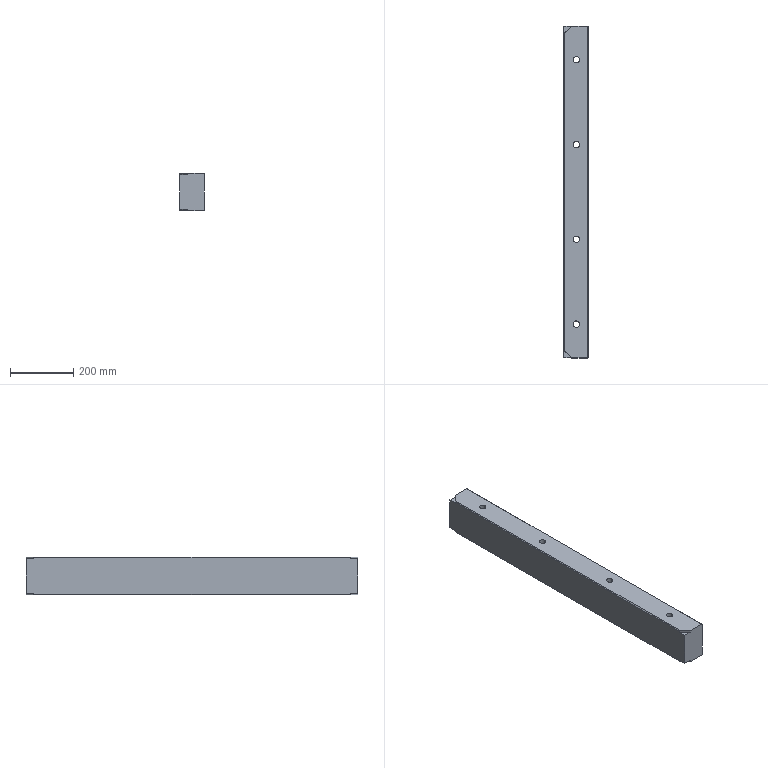Part | STEP file | 4-20.sldasm-Part-330 | 1 solid | 26 faces | box 78 x 1050 x 120 mm | volume 9659306 mm3 | plane 18 | cylinder 8 | commonest cylinder face diameters 19.842 x8
STEP:
#1=CARTESIAN_POINT('',(-175.079,-418.,-140.));
#2=VERTEX_POINT('',#1);
#3=CARTESIAN_POINT('',(-194.921,-418.,-140.));
#4=VERTEX_POINT('',#3);
#5=CARTESIAN_POINT('',(-185.,-418.,-140.));
#6=DIRECTION('',(0.,0.,-1.));
#7=DIRECTION('',(-1.,0.,0.));
#8=AXIS2_PLACEMENT_3D('',#5,#6,#7);
#9=CIRCLE('',#8,9.921);
#10=EDGE_CURVE('',#2,#4,#9,.T.);
#11=ORIENTED_EDGE('',*,*,#10,.T.);
#12=CARTESIAN_POINT('',(-194.921,-418.,-20.));
#13=VERTEX_POINT('',#12);
#14=CARTESIAN_POINT('',(-194.921,-418.,-160.701));
#15=DIRECTION('',(0.,0.,1.));
#16=VECTOR('',#15,1000.);
#17=LINE('',#14,#16);
#18=EDGE_CURVE('',#4,#13,#17,.T.);
#19=ORIENTED_EDGE('',*,*,#18,.T.);
#20=CARTESIAN_POINT('',(-175.079,-418.,-20.));
#21=VERTEX_POINT('',#20);
#22=CARTESIAN_POINT('',(-185.,-418.,-20.));
#23=DIRECTION('',(0.,0.,-1.));
#24=DIRECTION('',(-1.,0.,0.));
#25=AXIS2_PLACEMENT_3D('',#22,#23,#24);
#26=CIRCLE('',#25,9.921);
#27=EDGE_CURVE('',#21,#13,#26,.T.);
#28=ORIENTED_EDGE('',*,*,#27,.F.);
#29=CARTESIAN_POINT('',(-175.079,-418.,-160.701));
#30=DIRECTION('',(0.,0.,1.));
#31=VECTOR('',#30,1000.);
#32=LINE('',#29,#31);
#33=EDGE_CURVE('',#2,#21,#32,.T.);
#34=ORIENTED_EDGE('',*,*,#33,.F.);
#35=EDGE_LOOP('',(#11,#19,#28,#34));
#36=FACE_OUTER_BOUND('',#35,.T.);
#37=CARTESIAN_POINT('',(-185.,-418.,-160.701));
#38=DIRECTION('',(0.,0.,1.));
#39=DIRECTION('',(1.,0.,0.));
#40=AXIS2_PLACEMENT_3D('',#37,#38,#39);
#41=CYLINDRICAL_SURFACE('',#40,9.921);
#42=ADVANCED_FACE('',(#36),#41,.F.);
#43=CARTESIAN_POINT('',(-175.079,-150.,-140.));
#44=VERTEX_POINT('',#43);
#45=CARTESIAN_POINT('',(-194.921,-150.,-140.));
#46=VERTEX_POINT('',#45);
#47=CARTESIAN_POINT('',(-185.,-150.,-140.));
#48=DIRECTION('',(0.,0.,-1.));
#49=DIRECTION('',(-1.,0.,0.));
#50=AXIS2_PLACEMENT_3D('',#47,#48,#49);
#51=CIRCLE('',#50,9.921);
#52=EDGE_CURVE('',#44,#46,#51,.T.);
#53=ORIENTED_EDGE('',*,*,#52,.T.);
#54=CARTESIAN_POINT('',(-194.921,-150.,-20.));
#55=VERTEX_POINT('',#54);
#56=CARTESIAN_POINT('',(-194.921,-150.,-160.701));
#57=DIRECTION('',(0.,0.,1.));
#58=VECTOR('',#57,1000.);
#59=LINE('',#56,#58);
#60=EDGE_CURVE('',#46,#55,#59,.T.);
#61=ORIENTED_EDGE('',*,*,#60,.T.);
#62=CARTESIAN_POINT('',(-175.079,-150.,-20.));
#63=VERTEX_POINT('',#62);
#64=CARTESIAN_POINT('',(-185.,-150.,-20.));
#65=DIRECTION('',(0.,0.,-1.));
#66=DIRECTION('',(-1.,0.,0.));
#67=AXIS2_PLACEMENT_3D('',#64,#65,#66);
#68=CIRCLE('',#67,9.921);
#69=EDGE_CURVE('',#63,#55,#68,.T.);
#70=ORIENTED_EDGE('',*,*,#69,.F.);
#71=CARTESIAN_POINT('',(-175.079,-150.,-160.701));
#72=DIRECTION('',(0.,0.,1.));
#73=VECTOR('',#72,1000.);
#74=LINE('',#71,#73);
#75=EDGE_CURVE('',#44,#63,#74,.T.);
#76=ORIENTED_EDGE('',*,*,#75,.F.);
#77=EDGE_LOOP('',(#53,#61,#70,#76));
#78=FACE_OUTER_BOUND('',#77,.T.);
#79=CARTESIAN_POINT('',(-185.,-150.,-160.701));
#80=DIRECTION('',(0.,0.,1.));
#81=DIRECTION('',(1.,0.,0.));
#82=AXIS2_PLACEMENT_3D('',#79,#80,#81);
#83=CYLINDRICAL_SURFACE('',#82,9.921);
#84=ADVANCED_FACE('',(#78),#83,.F.);
#85=CARTESIAN_POINT('',(-175.079,150.,-140.));
#86=VERTEX_POINT('',#85);
#87=CARTESIAN_POINT('',(-194.921,150.,-140.));
#88=VERTEX_POINT('',#87);
#89=CARTESIAN_POINT('',(-185.,150.,-140.));
#90=DIRECTION('',(0.,0.,-1.));
#91=DIRECTION('',(-1.,0.,0.));
#92=AXIS2_PLACEMENT_3D('',#89,#90,#91);
#93=CIRCLE('',#92,9.921);
#94=EDGE_CURVE('',#86,#88,#93,.T.);
#95=ORIENTED_EDGE('',*,*,#94,.T.);
#96=CARTESIAN_POINT('',(-194.921,150.,-20.));
#97=VERTEX_POINT('',#96);
#98=CARTESIAN_POINT('',(-194.921,150.,-160.701));
#99=DIRECTION('',(0.,0.,1.));
#100=VECTOR('',#99,1000.);
#101=LINE('',#98,#100);
#102=EDGE_CURVE('',#88,#97,#101,.T.);
#103=ORIENTED_EDGE('',*,*,#102,.T.);
#104=CARTESIAN_POINT('',(-175.079,150.,-20.));
#105=VERTEX_POINT('',#104);
#106=CARTESIAN_POINT('',(-185.,150.,-20.));
#107=DIRECTION('',(0.,0.,-1.));
#108=DIRECTION('',(-1.,0.,0.));
#109=AXIS2_PLACEMENT_3D('',#106,#107,#108);
#110=CIRCLE('',#109,9.921);
#111=EDGE_CURVE('',#105,#97,#110,.T.);
#112=ORIENTED_EDGE('',*,*,#111,.F.);
#113=CARTESIAN_POINT('',(-175.079,150.,-160.701));
#114=DIRECTION('',(0.,0.,1.));
#115=VECTOR('',#114,1000.);
#116=LINE('',#113,#115);
#117=EDGE_CURVE('',#86,#105,#116,.T.);
#118=ORIENTED_EDGE('',*,*,#117,.F.);
#119=EDGE_LOOP('',(#95,#103,#112,#118));
#120=FACE_OUTER_BOUND('',#119,.T.);
#121=CARTESIAN_POINT('',(-185.,150.,-160.701));
#122=DIRECTION('',(0.,0.,1.));
#123=DIRECTION('',(1.,0.,0.));
#124=AXIS2_PLACEMENT_3D('',#121,#122,#123);
#125=CYLINDRICAL_SURFACE('',#124,9.921);
#126=ADVANCED_FACE('',(#120),#125,.F.);
#127=CARTESIAN_POINT('',(-175.079,418.,-140.));
#128=VERTEX_POINT('',#127);
#129=CARTESIAN_POINT('',(-194.921,418.,-140.));
#130=VERTEX_POINT('',#129);
#131=CARTESIAN_POINT('',(-185.,418.,-140.));
#132=DIRECTION('',(0.,0.,-1.));
#133=DIRECTION('',(-1.,0.,0.));
#134=AXIS2_PLACEMENT_3D('',#131,#132,#133);
#135=CIRCLE('',#134,9.921);
#136=EDGE_CURVE('',#128,#130,#135,.T.);
#137=ORIENTED_EDGE('',*,*,#136,.T.);
#138=CARTESIAN_POINT('',(-194.921,418.,-20.));
#139=VERTEX_POINT('',#138);
#140=CARTESIAN_POINT('',(-194.921,418.,-160.701));
#141=DIRECTION('',(0.,0.,1.));
#142=VECTOR('',#141,1000.);
#143=LINE('',#140,#142);
#144=EDGE_CURVE('',#130,#139,#143,.T.);
#145=ORIENTED_EDGE('',*,*,#144,.T.);
#146=CARTESIAN_POINT('',(-175.079,418.,-20.));
#147=VERTEX_POINT('',#146);
#148=CARTESIAN_POINT('',(-185.,418.,-20.));
#149=DIRECTION('',(0.,0.,-1.));
#150=DIRECTION('',(-1.,0.,0.));
#151=AXIS2_PLACEMENT_3D('',#148,#149,#150);
#152=CIRCLE('',#151,9.921);
#153=EDGE_CURVE('',#147,#139,#152,.T.);
#154=ORIENTED_EDGE('',*,*,#153,.F.);
#155=CARTESIAN_POINT('',(-175.079,418.,-160.701));
#156=DIRECTION('',(0.,0.,1.));
#157=VECTOR('',#156,1000.);
#158=LINE('',#155,#157);
#159=EDGE_CURVE('',#128,#147,#158,.T.);
#160=ORIENTED_EDGE('',*,*,#159,.F.);
#161=EDGE_LOOP('',(#137,#145,#154,#160));
#162=FACE_OUTER_BOUND('',#161,.T.);
#163=CARTESIAN_POINT('',(-185.,418.,-160.701));
#164=DIRECTION('',(0.,0.,1.));
#165=DIRECTION('',(1.,0.,0.));
#166=AXIS2_PLACEMENT_3D('',#163,#164,#165);
#167=CYLINDRICAL_SURFACE('',#166,9.921);
#168=ADVANCED_FACE('',(#162),#167,.F.);
#169=CARTESIAN_POINT('',(-222.5,502.601,-140.));
#170=VERTEX_POINT('',#169);
#171=CARTESIAN_POINT('',(-222.5,-502.601,-140.));
#172=VERTEX_POINT('',#171);
#173=CARTESIAN_POINT('',(-222.5,0.,-140.));
#174=DIRECTION('',(0.,-1.,0.));
#175=VECTOR('',#174,1000.);
#176=LINE('',#173,#175);
#177=EDGE_CURVE('',#170,#172,#176,.T.);
#178=ORIENTED_EDGE('',*,*,#177,.T.);
#179=CARTESIAN_POINT('',(-225.,-500.101,-137.5));
#180=VERTEX_POINT('',#179);
#181=CARTESIAN_POINT('',(-390.034,-335.067,27.534));
#182=DIRECTION('',(-0.5774,0.5774,0.5774));
#183=VECTOR('',#182,1000.);
#184=LINE('',#181,#183);
#185=EDGE_CURVE('',#172,#180,#184,.T.);
#186=ORIENTED_EDGE('',*,*,#185,.T.);
#187=CARTESIAN_POINT('',(-225.,500.101,-137.5));
#188=VERTEX_POINT('',#187);
#189=CARTESIAN_POINT('',(-225.,0.,-137.5));
#190=DIRECTION('',(0.,1.,0.));
#191=VECTOR('',#190,1000.);
#192=LINE('',#189,#191);
#193=EDGE_CURVE('',#180,#188,#192,.T.);
#194=ORIENTED_EDGE('',*,*,#193,.T.);
#195=CARTESIAN_POINT('',(-390.034,335.067,27.534));
#196=DIRECTION('',(0.5774,0.5774,-0.5774));
#197=VECTOR('',#196,1000.);
#198=LINE('',#195,#197);
#199=EDGE_CURVE('',#188,#170,#198,.T.);
#200=ORIENTED_EDGE('',*,*,#199,.T.);
#201=EDGE_LOOP('',(#178,#186,#194,#200));
#202=FACE_OUTER_BOUND('',#201,.T.);
#203=CARTESIAN_POINT('',(-222.5,0.,-140.));
#204=DIRECTION('',(0.7071,0.,0.7071));
#205=DIRECTION('',(-0.7071,0.,0.7071));
#206=AXIS2_PLACEMENT_3D('',#203,#204,#205);
#207=PLANE('',#206);
#208=ADVANCED_FACE('',(#202),#207,.F.);
#209=CARTESIAN_POINT('',(-225.,-500.101,-134.));
#210=VERTEX_POINT('',#209);
#211=CARTESIAN_POINT('',(-225.,-500.101,-140.));
#212=DIRECTION('',(0.,0.,1.));
#213=VECTOR('',#212,1000.);
#214=LINE('',#211,#213);
#215=EDGE_CURVE('',#180,#210,#214,.T.);
#216=ORIENTED_EDGE('',*,*,#215,.T.);
#217=CARTESIAN_POINT('',(-225.,-525.,-134.));
#218=VERTEX_POINT('',#217);
#219=CARTESIAN_POINT('',(-225.,-510.,-134.));
#220=DIRECTION('',(0.,-1.,0.));
#221=VECTOR('',#220,1000.);
#222=LINE('',#219,#221);
#223=EDGE_CURVE('',#210,#218,#222,.T.);
#224=ORIENTED_EDGE('',*,*,#223,.T.);
#225=CARTESIAN_POINT('',(-225.,-525.,-26.));
#226=VERTEX_POINT('',#225);
#227=CARTESIAN_POINT('',(-225.,-525.,298.5));
#228=DIRECTION('',(0.,0.,1.));
#229=VECTOR('',#228,1000.);
#230=LINE('',#227,#229);
#231=EDGE_CURVE('',#218,#226,#230,.T.);
#232=ORIENTED_EDGE('',*,*,#231,.T.);
#233=CARTESIAN_POINT('',(-225.,-500.101,-26.));
#234=VERTEX_POINT('',#233);
#235=CARTESIAN_POINT('',(-225.,-510.,-26.));
#236=DIRECTION('',(0.,-1.,0.));
#237=VECTOR('',#236,1000.);
#238=LINE('',#235,#237);
#239=EDGE_CURVE('',#234,#226,#238,.T.);
#240=ORIENTED_EDGE('',*,*,#239,.F.);
#241=CARTESIAN_POINT('',(-225.,-500.101,-22.5));
#242=VERTEX_POINT('',#241);
#243=CARTESIAN_POINT('',(-225.,-500.101,-26.));
#244=DIRECTION('',(0.,0.,1.));
#245=VECTOR('',#244,1000.);
#246=LINE('',#243,#245);
#247=EDGE_CURVE('',#234,#242,#246,.T.);
#248=ORIENTED_EDGE('',*,*,#247,.T.);
#249=CARTESIAN_POINT('',(-225.,500.101,-22.5));
#250=VERTEX_POINT('',#249);
#251=CARTESIAN_POINT('',(-225.,-500.,-22.5));
#252=DIRECTION('',(0.,-1.,0.));
#253=VECTOR('',#252,1000.);
#254=LINE('',#251,#253);
#255=EDGE_CURVE('',#250,#242,#254,.T.);
#256=ORIENTED_EDGE('',*,*,#255,.F.);
#257=CARTESIAN_POINT('',(-225.,500.101,-26.));
#258=VERTEX_POINT('',#257);
#259=CARTESIAN_POINT('',(-225.,500.101,-26.));
#260=DIRECTION('',(0.,0.,1.));
#261=VECTOR('',#260,1000.);
#262=LINE('',#259,#261);
#263=EDGE_CURVE('',#258,#250,#262,.T.);
#264=ORIENTED_EDGE('',*,*,#263,.F.);
#265=CARTESIAN_POINT('',(-225.,525.,-26.));
#266=VERTEX_POINT('',#265);
#267=CARTESIAN_POINT('',(-225.,510.,-26.));
#268=DIRECTION('',(0.,1.,0.));
#269=VECTOR('',#268,1000.);
#270=LINE('',#267,#269);
#271=EDGE_CURVE('',#258,#266,#270,.T.);
#272=ORIENTED_EDGE('',*,*,#271,.T.);
#273=CARTESIAN_POINT('',(-225.,525.,-134.));
#274=VERTEX_POINT('',#273);
#275=CARTESIAN_POINT('',(-225.,525.,298.5));
#276=DIRECTION('',(0.,0.,-1.));
#277=VECTOR('',#276,1000.);
#278=LINE('',#275,#277);
#279=EDGE_CURVE('',#266,#274,#278,.T.);
#280=ORIENTED_EDGE('',*,*,#279,.T.);
#281=CARTESIAN_POINT('',(-225.,500.101,-134.));
#282=VERTEX_POINT('',#281);
#283=CARTESIAN_POINT('',(-225.,510.,-134.));
#284=DIRECTION('',(0.,1.,0.));
#285=VECTOR('',#284,1000.);
#286=LINE('',#283,#285);
#287=EDGE_CURVE('',#282,#274,#286,.T.);
#288=ORIENTED_EDGE('',*,*,#287,.F.);
#289=CARTESIAN_POINT('',(-225.,500.101,-140.));
#290=DIRECTION('',(0.,0.,1.));
#291=VECTOR('',#290,1000.);
#292=LINE('',#289,#291);
#293=EDGE_CURVE('',#188,#282,#292,.T.);
#294=ORIENTED_EDGE('',*,*,#293,.F.);
#295=ORIENTED_EDGE('',*,*,#193,.F.);
#296=EDGE_LOOP('',(#216,#224,#232,#240,#248,#256,#264,#272,#280,#288,#294,#295));
#297=FACE_OUTER_BOUND('',#296,.T.);
#298=CARTESIAN_POINT('',(-225.,0.,298.5));
#299=DIRECTION('',(-1.,0.,0.));
#300=DIRECTION('',(0.,0.,-1.));
#301=AXIS2_PLACEMENT_3D('',#298,#299,#300);
#302=PLANE('',#301);
#303=ADVANCED_FACE('',(#297),#302,.T.);
#304=ORIENTED_EDGE('',*,*,#231,.F.);
#305=CARTESIAN_POINT('',(-200.101,-525.,-134.));
#306=VERTEX_POINT('',#305);
#307=CARTESIAN_POINT('',(-225.,-525.,-134.));
#308=DIRECTION('',(1.,0.,0.));
#309=VECTOR('',#308,1000.);
#310=LINE('',#307,#309);
#311=EDGE_CURVE('',#218,#306,#310,.T.);
#312=ORIENTED_EDGE('',*,*,#311,.T.);
#313=CARTESIAN_POINT('',(-200.101,-525.,-140.));
#314=VERTEX_POINT('',#313);
#315=CARTESIAN_POINT('',(-200.101,-525.,-140.));
#316=DIRECTION('',(0.,0.,1.));
#317=VECTOR('',#316,1000.);
#318=LINE('',#315,#317);
#319=EDGE_CURVE('',#314,#306,#318,.T.);
#320=ORIENTED_EDGE('',*,*,#319,.F.);
#321=CARTESIAN_POINT('',(-149.5,-525.,-140.));
#322=VERTEX_POINT('',#321);
#323=CARTESIAN_POINT('',(-187.5,-525.,-140.));
#324=DIRECTION('',(-1.,0.,0.));
#325=VECTOR('',#324,1000.);
#326=LINE('',#323,#325);
#327=EDGE_CURVE('',#322,#314,#326,.T.);
#328=ORIENTED_EDGE('',*,*,#327,.F.);
#329=CARTESIAN_POINT('',(-147.,-525.,-137.5));
#330=VERTEX_POINT('',#329);
#331=CARTESIAN_POINT('',(-149.5,-525.,-140.));
#332=DIRECTION('',(-0.7071,0.,-0.7071));
#333=VECTOR('',#332,1000.);
#334=LINE('',#331,#333);
#335=EDGE_CURVE('',#330,#322,#334,.T.);
#336=ORIENTED_EDGE('',*,*,#335,.F.);
#337=CARTESIAN_POINT('',(-147.,-525.,-22.5));
#338=VERTEX_POINT('',#337);
#339=CARTESIAN_POINT('',(-147.,-525.,-117.5));
#340=DIRECTION('',(0.,0.,-1.));
#341=VECTOR('',#340,1000.);
#342=LINE('',#339,#341);
#343=EDGE_CURVE('',#338,#330,#342,.T.);
#344=ORIENTED_EDGE('',*,*,#343,.F.);
#345=CARTESIAN_POINT('',(-149.5,-525.,-20.));
#346=VERTEX_POINT('',#345);
#347=CARTESIAN_POINT('',(-147.,-525.,-22.5));
#348=DIRECTION('',(0.7071,0.,-0.7071));
#349=VECTOR('',#348,1000.);
#350=LINE('',#347,#349);
#351=EDGE_CURVE('',#346,#338,#350,.T.);
#352=ORIENTED_EDGE('',*,*,#351,.F.);
#353=CARTESIAN_POINT('',(-200.101,-525.,-20.));
#354=VERTEX_POINT('',#353);
#355=CARTESIAN_POINT('',(-222.5,-525.,-20.));
#356=DIRECTION('',(-1.,0.,0.));
#357=VECTOR('',#356,1000.);
#358=LINE('',#355,#357);
#359=EDGE_CURVE('',#346,#354,#358,.T.);
#360=ORIENTED_EDGE('',*,*,#359,.T.);
#361=CARTESIAN_POINT('',(-200.101,-525.,-26.));
#362=VERTEX_POINT('',#361);
#363=CARTESIAN_POINT('',(-200.101,-525.,-26.));
#364=DIRECTION('',(0.,0.,1.));
#365=VECTOR('',#364,1000.);
#366=LINE('',#363,#365);
#367=EDGE_CURVE('',#362,#354,#366,.T.);
#368=ORIENTED_EDGE('',*,*,#367,.F.);
#369=CARTESIAN_POINT('',(-225.,-525.,-26.));
#370=DIRECTION('',(1.,0.,0.));
#371=VECTOR('',#370,1000.);
#372=LINE('',#369,#371);
#373=EDGE_CURVE('',#226,#362,#372,.T.);
#374=ORIENTED_EDGE('',*,*,#373,.F.);
#375=EDGE_LOOP('',(#304,#312,#320,#328,#336,#344,#352,#360,#368,#374));
#376=FACE_OUTER_BOUND('',#375,.T.);
#377=CARTESIAN_POINT('',(-247.5,-525.,679.));
#378=DIRECTION('',(0.,-1.,0.));
#379=DIRECTION('',(0.,0.,-1.));
#380=AXIS2_PLACEMENT_3D('',#377,#378,#379);
#381=PLANE('',#380);
#382=ADVANCED_FACE('',(#376),#381,.T.);
#383=ORIENTED_EDGE('',*,*,#136,.F.);
#384=CARTESIAN_POINT('',(-185.,418.,-140.));
#385=DIRECTION('',(0.,0.,-1.));
#386=DIRECTION('',(-1.,0.,0.));
#387=AXIS2_PLACEMENT_3D('',#384,#385,#386);
#388=CIRCLE('',#387,9.921);
#389=EDGE_CURVE('',#130,#128,#388,.T.);
#390=ORIENTED_EDGE('',*,*,#389,.F.);
#391=EDGE_LOOP('',(#383,#390));
#392=FACE_BOUND('',#391,.T.);
#393=ORIENTED_EDGE('',*,*,#94,.F.);
#394=CARTESIAN_POINT('',(-185.,150.,-140.));
#395=DIRECTION('',(0.,0.,-1.));
#396=DIRECTION('',(-1.,0.,0.));
#397=AXIS2_PLACEMENT_3D('',#394,#395,#396);
#398=CIRCLE('',#397,9.921);
#399=EDGE_CURVE('',#88,#86,#398,.T.);
#400=ORIENTED_EDGE('',*,*,#399,.F.);
#401=EDGE_LOOP('',(#393,#400));
#402=FACE_BOUND('',#401,.T.);
#403=ORIENTED_EDGE('',*,*,#52,.F.);
#404=CARTESIAN_POINT('',(-185.,-150.,-140.));
#405=DIRECTION('',(0.,0.,-1.));
#406=DIRECTION('',(-1.,0.,0.));
#407=AXIS2_PLACEMENT_3D('',#404,#405,#406);
#408=CIRCLE('',#407,9.921);
#409=EDGE_CURVE('',#46,#44,#408,.T.);
#410=ORIENTED_EDGE('',*,*,#409,.F.);
#411=EDGE_LOOP('',(#403,#410));
#412=FACE_BOUND('',#411,.T.);
#413=ORIENTED_EDGE('',*,*,#10,.F.);
#414=CARTESIAN_POINT('',(-185.,-418.,-140.));
#415=DIRECTION('',(0.,0.,-1.));
#416=DIRECTION('',(-1.,0.,0.));
#417=AXIS2_PLACEMENT_3D('',#414,#415,#416);
#418=CIRCLE('',#417,9.921);
#419=EDGE_CURVE('',#4,#2,#418,.T.);
#420=ORIENTED_EDGE('',*,*,#419,.F.);
#421=EDGE_LOOP('',(#413,#420));
#422=FACE_BOUND('',#421,.T.);
#423=ORIENTED_EDGE('',*,*,#327,.T.);
#424=CARTESIAN_POINT('',(-205.05,-520.05,-140.));
#425=DIRECTION('',(-0.7071,0.7071,0.));
#426=VECTOR('',#425,1000.);
#427=LINE('',#424,#426);
#428=EDGE_CURVE('',#314,#172,#427,.T.);
#429=ORIENTED_EDGE('',*,*,#428,.T.);
#430=ORIENTED_EDGE('',*,*,#177,.F.);
#431=CARTESIAN_POINT('',(-200.101,525.,-140.));
#432=VERTEX_POINT('',#431);
#433=CARTESIAN_POINT('',(-205.05,520.05,-140.));
#434=DIRECTION('',(-0.7071,-0.7071,0.));
#435=VECTOR('',#434,1000.);
#436=LINE('',#433,#435);
#437=EDGE_CURVE('',#432,#170,#436,.T.);
#438=ORIENTED_EDGE('',*,*,#437,.F.);
#439=CARTESIAN_POINT('',(-149.5,525.,-140.));
#440=VERTEX_POINT('',#439);
#441=CARTESIAN_POINT('',(-187.5,525.,-140.));
#442=DIRECTION('',(1.,0.,0.));
#443=VECTOR('',#442,1000.);
#444=LINE('',#441,#443);
#445=EDGE_CURVE('',#432,#440,#444,.T.);
#446=ORIENTED_EDGE('',*,*,#445,.T.);
#447=CARTESIAN_POINT('',(-149.5,0.,-140.));
#448=DIRECTION('',(0.,1.,0.));
#449=VECTOR('',#448,1000.);
#450=LINE('',#447,#449);
#451=EDGE_CURVE('',#322,#440,#450,.T.);
#452=ORIENTED_EDGE('',*,*,#451,.F.);
#453=EDGE_LOOP('',(#423,#429,#430,#438,#446,#452));
#454=FACE_OUTER_BOUND('',#453,.T.);
#455=CARTESIAN_POINT('',(-187.5,0.,-140.));
#456=DIRECTION('',(0.,0.,-1.));
#457=DIRECTION('',(1.,0.,0.));
#458=AXIS2_PLACEMENT_3D('',#455,#456,#457);
#459=PLANE('',#458);
#460=ADVANCED_FACE('',(#392,#402,#412,#422,#454),#459,.T.);
#461=ORIENTED_EDGE('',*,*,#255,.T.);
#462=CARTESIAN_POINT('',(-222.5,-502.601,-20.));
#463=VERTEX_POINT('',#462);
#464=CARTESIAN_POINT('',(-390.034,-335.067,-187.534));
#465=DIRECTION('',(0.5774,-0.5774,0.5774));
#466=VECTOR('',#465,1000.);
#467=LINE('',#464,#466);
#468=EDGE_CURVE('',#242,#463,#467,.T.);
#469=ORIENTED_EDGE('',*,*,#468,.T.);
#470=CARTESIAN_POINT('',(-222.5,502.601,-20.));
#471=VERTEX_POINT('',#470);
#472=CARTESIAN_POINT('',(-222.5,500.,-20.));
#473=DIRECTION('',(0.,1.,0.));
#474=VECTOR('',#473,1000.);
#475=LINE('',#472,#474);
#476=EDGE_CURVE('',#463,#471,#475,.T.);
#477=ORIENTED_EDGE('',*,*,#476,.T.);
#478=CARTESIAN_POINT('',(-390.034,335.067,-187.534));
#479=DIRECTION('',(-0.5774,-0.5774,-0.5774));
#480=VECTOR('',#479,1000.);
#481=LINE('',#478,#480);
#482=EDGE_CURVE('',#471,#250,#481,.T.);
#483=ORIENTED_EDGE('',*,*,#482,.T.);
#484=EDGE_LOOP('',(#461,#469,#477,#483));
#485=FACE_OUTER_BOUND('',#484,.T.);
#486=CARTESIAN_POINT('',(-222.5,0.,-20.));
#487=DIRECTION('',(-0.7071,0.,0.7071));
#488=DIRECTION('',(-0.7071,0.,-0.7071));
#489=AXIS2_PLACEMENT_3D('',#486,#487,#488);
#490=PLANE('',#489);
#491=ADVANCED_FACE('',(#485),#490,.T.);
#492=ORIENTED_EDGE('',*,*,#153,.T.);
#493=CARTESIAN_POINT('',(-185.,418.,-20.));
#494=DIRECTION('',(0.,0.,-1.));
#495=DIRECTION('',(-1.,0.,0.));
#496=AXIS2_PLACEMENT_3D('',#493,#494,#495);
#497=CIRCLE('',#496,9.921);
#498=EDGE_CURVE('',#139,#147,#497,.T.);
#499=ORIENTED_EDGE('',*,*,#498,.T.);
#500=EDGE_LOOP('',(#492,#499));
#501=FACE_BOUND('',#500,.T.);
#502=ORIENTED_EDGE('',*,*,#111,.T.);
#503=CARTESIAN_POINT('',(-185.,150.,-20.));
#504=DIRECTION('',(0.,0.,-1.));
#505=DIRECTION('',(-1.,0.,0.));
#506=AXIS2_PLACEMENT_3D('',#503,#504,#505);
#507=CIRCLE('',#506,9.921);
#508=EDGE_CURVE('',#97,#105,#507,.T.);
#509=ORIENTED_EDGE('',*,*,#508,.T.);
#510=EDGE_LOOP('',(#502,#509));
#511=FACE_BOUND('',#510,.T.);
#512=ORIENTED_EDGE('',*,*,#69,.T.);
#513=CARTESIAN_POINT('',(-185.,-150.,-20.));
#514=DIRECTION('',(0.,0.,-1.));
#515=DIRECTION('',(-1.,0.,0.));
#516=AXIS2_PLACEMENT_3D('',#513,#514,#515);
#517=CIRCLE('',#516,9.921);
#518=EDGE_CURVE('',#55,#63,#517,.T.);
#519=ORIENTED_EDGE('',*,*,#518,.T.);
#520=EDGE_LOOP('',(#512,#519));
#521=FACE_BOUND('',#520,.T.);
#522=ORIENTED_EDGE('',*,*,#27,.T.);
#523=CARTESIAN_POINT('',(-185.,-418.,-20.));
#524=DIRECTION('',(0.,0.,-1.));
#525=DIRECTION('',(-1.,0.,0.));
#526=AXIS2_PLACEMENT_3D('',#523,#524,#525);
#527=CIRCLE('',#526,9.921);
#528=EDGE_CURVE('',#13,#21,#527,.T.);
#529=ORIENTED_EDGE('',*,*,#528,.T.);
#530=EDGE_LOOP('',(#522,#529));
#531=FACE_BOUND('',#530,.T.);
#532=CARTESIAN_POINT('',(-205.05,-520.05,-20.));
#533=DIRECTION('',(-0.7071,0.7071,0.));
#534=VECTOR('',#533,1000.);
#535=LINE('',#532,#534);
#536=EDGE_CURVE('',#354,#463,#535,.T.);
#537=ORIENTED_EDGE('',*,*,#536,.F.);
#538=ORIENTED_EDGE('',*,*,#359,.F.);
#539=CARTESIAN_POINT('',(-149.5,525.,-20.));
#540=VERTEX_POINT('',#539);
#541=CARTESIAN_POINT('',(-149.5,-500.,-20.));
#542=DIRECTION('',(0.,-1.,0.));
#543=VECTOR('',#542,1000.);
#544=LINE('',#541,#543);
#545=EDGE_CURVE('',#540,#346,#544,.T.);
#546=ORIENTED_EDGE('',*,*,#545,.F.);
#547=CARTESIAN_POINT('',(-200.101,525.,-20.));
#548=VERTEX_POINT('',#547);
#549=CARTESIAN_POINT('',(-222.5,525.,-20.));
#550=DIRECTION('',(1.,0.,0.));
#551=VECTOR('',#550,1000.);
#552=LINE('',#549,#551);
#553=EDGE_CURVE('',#548,#540,#552,.T.);
#554=ORIENTED_EDGE('',*,*,#553,.F.);
#555=CARTESIAN_POINT('',(-205.05,520.05,-20.));
#556=DIRECTION('',(-0.7071,-0.7071,0.));
#557=VECTOR('',#556,1000.);
#558=LINE('',#555,#557);
#559=EDGE_CURVE('',#548,#471,#558,.T.);
#560=ORIENTED_EDGE('',*,*,#559,.T.);
#561=ORIENTED_EDGE('',*,*,#476,.F.);
#562=EDGE_LOOP('',(#537,#538,#546,#554,#560,#561));
#563=FACE_OUTER_BOUND('',#562,.T.);
#564=CARTESIAN_POINT('',(-222.5,0.,-20.));
#565=DIRECTION('',(0.,0.,-1.));
#566=DIRECTION('',(1.,0.,0.));
#567=AXIS2_PLACEMENT_3D('',#564,#565,#566);
#568=PLANE('',#567);
#569=ADVANCED_FACE('',(#501,#511,#521,#531,#563),#568,.F.);
#570=CARTESIAN_POINT('',(-200.101,525.,-134.));
#571=VERTEX_POINT('',#570);
#572=CARTESIAN_POINT('',(-225.,525.,-134.));
#573=DIRECTION('',(1.,0.,0.));
#574=VECTOR('',#573,1000.);
#575=LINE('',#572,#574);
#576=EDGE_CURVE('',#274,#571,#575,.T.);
#577=ORIENTED_EDGE('',*,*,#576,.F.);
#578=ORIENTED_EDGE('',*,*,#279,.F.);
#579=CARTESIAN_POINT('',(-200.101,525.,-26.));
#580=VERTEX_POINT('',#579);
#581=CARTESIAN_POINT('',(-225.,525.,-26.));
#582=DIRECTION('',(1.,0.,0.));
#583=VECTOR('',#582,1000.);
#584=LINE('',#581,#583);
#585=EDGE_CURVE('',#266,#580,#584,.T.);
#586=ORIENTED_EDGE('',*,*,#585,.T.);
#587=CARTESIAN_POINT('',(-200.101,525.,-26.));
#588=DIRECTION('',(0.,0.,1.));
#589=VECTOR('',#588,1000.);
#590=LINE('',#587,#589);
#591=EDGE_CURVE('',#580,#548,#590,.T.);
#592=ORIENTED_EDGE('',*,*,#591,.T.);
#593=ORIENTED_EDGE('',*,*,#553,.T.);
#594=CARTESIAN_POINT('',(-147.,525.,-22.5));
#595=VERTEX_POINT('',#594);
#596=CARTESIAN_POINT('',(-147.,525.,-22.5));
#597=DIRECTION('',(-0.7071,0.,0.7071));
#598=VECTOR('',#597,1000.);
#599=LINE('',#596,#598);
#600=EDGE_CURVE('',#595,#540,#599,.T.);
#601=ORIENTED_EDGE('',*,*,#600,.F.);
#602=CARTESIAN_POINT('',(-147.,525.,-137.5));
#603=VERTEX_POINT('',#602);
#604=CARTESIAN_POINT('',(-147.,525.,-117.5));
#605=DIRECTION('',(0.,0.,1.));
#606=VECTOR('',#605,1000.);
#607=LINE('',#604,#606);
#608=EDGE_CURVE('',#603,#595,#607,.T.);
#609=ORIENTED_EDGE('',*,*,#608,.F.);
#610=CARTESIAN_POINT('',(-149.5,525.,-140.));
#611=DIRECTION('',(0.7071,0.,0.7071));
#612=VECTOR('',#611,1000.);
#613=LINE('',#610,#612);
#614=EDGE_CURVE('',#440,#603,#613,.T.);
#615=ORIENTED_EDGE('',*,*,#614,.F.);
#616=ORIENTED_EDGE('',*,*,#445,.F.);
#617=CARTESIAN_POINT('',(-200.101,525.,-140.));
#618=DIRECTION('',(0.,0.,1.));
#619=VECTOR('',#618,1000.);
#620=LINE('',#617,#619);
#621=EDGE_CURVE('',#432,#571,#620,.T.);
#622=ORIENTED_EDGE('',*,*,#621,.T.);
#623=EDGE_LOOP('',(#577,#578,#586,#592,#593,#601,#609,#615,#616,#622));
#624=FACE_OUTER_BOUND('',#623,.T.);
#625=CARTESIAN_POINT('',(147.5,525.,679.));
#626=DIRECTION('',(0.,1.,0.));
#627=DIRECTION('',(0.,0.,1.));
#628=AXIS2_PLACEMENT_3D('',#625,#626,#627);
#629=PLANE('',#628);
#630=ADVANCED_FACE('',(#624),#629,.T.);
#631=ORIENTED_EDGE('',*,*,#608,.T.);
#632=CARTESIAN_POINT('',(-147.,500.,-22.5));
#633=DIRECTION('',(0.,1.,0.));
#634=VECTOR('',#633,1000.);
#635=LINE('',#632,#634);
#636=EDGE_CURVE('',#338,#595,#635,.T.);
#637=ORIENTED_EDGE('',*,*,#636,.F.);
#638=ORIENTED_EDGE('',*,*,#343,.T.);
#639=CARTESIAN_POINT('',(-147.,0.,-137.5));
#640=DIRECTION('',(0.,-1.,0.));
#641=VECTOR('',#640,1000.);
#642=LINE('',#639,#641);
#643=EDGE_CURVE('',#603,#330,#642,.T.);
#644=ORIENTED_EDGE('',*,*,#643,.F.);
#645=EDGE_LOOP('',(#631,#637,#638,#644));
#646=FACE_OUTER_BOUND('',#645,.T.);
#647=CARTESIAN_POINT('',(-147.,0.,-117.5));
#648=DIRECTION('',(1.,0.,0.));
#649=DIRECTION('',(0.,0.,1.));
#650=AXIS2_PLACEMENT_3D('',#647,#648,#649);
#651=PLANE('',#650);
#652=ADVANCED_FACE('',(#646),#651,.T.);
#653=ORIENTED_EDGE('',*,*,#335,.T.);
#654=ORIENTED_EDGE('',*,*,#451,.T.);
#655=ORIENTED_EDGE('',*,*,#614,.T.);
#656=ORIENTED_EDGE('',*,*,#643,.T.);
#657=EDGE_LOOP('',(#653,#654,#655,#656));
#658=FACE_OUTER_BOUND('',#657,.T.);
#659=CARTESIAN_POINT('',(-149.5,0.,-140.));
#660=DIRECTION('',(-0.7071,0.,0.7071));
#661=DIRECTION('',(-0.7071,0.,-0.7071));
#662=AXIS2_PLACEMENT_3D('',#659,#660,#661);
#663=PLANE('',#662);
#664=ADVANCED_FACE('',(#658),#663,.F.);
#665=ORIENTED_EDGE('',*,*,#351,.T.);
#666=ORIENTED_EDGE('',*,*,#636,.T.);
#667=ORIENTED_EDGE('',*,*,#600,.T.);
#668=ORIENTED_EDGE('',*,*,#545,.T.);
#669=EDGE_LOOP('',(#665,#666,#667,#668));
#670=FACE_OUTER_BOUND('',#669,.T.);
#671=CARTESIAN_POINT('',(-147.,0.,-22.5));
#672=DIRECTION('',(0.7071,0.,0.7071));
#673=DIRECTION('',(-0.7071,0.,0.7071));
#674=AXIS2_PLACEMENT_3D('',#671,#672,#673);
#675=PLANE('',#674);
#676=ADVANCED_FACE('',(#670),#675,.T.);
#677=ORIENTED_EDGE('',*,*,#144,.F.);
#678=ORIENTED_EDGE('',*,*,#389,.T.);
#679=ORIENTED_EDGE('',*,*,#159,.T.);
#680=ORIENTED_EDGE('',*,*,#498,.F.);
#681=EDGE_LOOP('',(#677,#678,#679,#680));
#682=FACE_OUTER_BOUND('',#681,.T.);
#683=CARTESIAN_POINT('',(-185.,418.,-160.701));
#684=DIRECTION('',(0.,0.,1.));
#685=DIRECTION('',(1.,0.,0.));
#686=AXIS2_PLACEMENT_3D('',#683,#684,#685);
#687=CYLINDRICAL_SURFACE('',#686,9.921);
#688=ADVANCED_FACE('',(#682),#687,.F.);
#689=ORIENTED_EDGE('',*,*,#102,.F.);
#690=ORIENTED_EDGE('',*,*,#399,.T.);
#691=ORIENTED_EDGE('',*,*,#117,.T.);
#692=ORIENTED_EDGE('',*,*,#508,.F.);
#693=EDGE_LOOP('',(#689,#690,#691,#692));
#694=FACE_OUTER_BOUND('',#693,.T.);
#695=CARTESIAN_POINT('',(-185.,150.,-160.701));
#696=DIRECTION('',(0.,0.,1.));
#697=DIRECTION('',(1.,0.,0.));
#698=AXIS2_PLACEMENT_3D('',#695,#696,#697);
#699=CYLINDRICAL_SURFACE('',#698,9.921);
#700=ADVANCED_FACE('',(#694),#699,.F.);
#701=ORIENTED_EDGE('',*,*,#60,.F.);
#702=ORIENTED_EDGE('',*,*,#409,.T.);
#703=ORIENTED_EDGE('',*,*,#75,.T.);
#704=ORIENTED_EDGE('',*,*,#518,.F.);
#705=EDGE_LOOP('',(#701,#702,#703,#704));
#706=FACE_OUTER_BOUND('',#705,.T.);
#707=CARTESIAN_POINT('',(-185.,-150.,-160.701));
#708=DIRECTION('',(0.,0.,1.));
#709=DIRECTION('',(1.,0.,0.));
#710=AXIS2_PLACEMENT_3D('',#707,#708,#709);
#711=CYLINDRICAL_SURFACE('',#710,9.921);
#712=ADVANCED_FACE('',(#706),#711,.F.);
#713=ORIENTED_EDGE('',*,*,#18,.F.);
#714=ORIENTED_EDGE('',*,*,#419,.T.);
#715=ORIENTED_EDGE('',*,*,#33,.T.);
#716=ORIENTED_EDGE('',*,*,#528,.F.);
#717=EDGE_LOOP('',(#713,#714,#715,#716));
#718=FACE_OUTER_BOUND('',#717,.T.);
#719=CARTESIAN_POINT('',(-185.,-418.,-160.701));
#720=DIRECTION('',(0.,0.,1.));
#721=DIRECTION('',(1.,0.,0.));
#722=AXIS2_PLACEMENT_3D('',#719,#720,#721);
#723=CYLINDRICAL_SURFACE('',#722,9.921);
#724=ADVANCED_FACE('',(#718),#723,.F.);
#725=ORIENTED_EDGE('',*,*,#559,.F.);
#726=ORIENTED_EDGE('',*,*,#591,.F.);
#727=CARTESIAN_POINT('',(-205.05,520.05,-26.));
#728=DIRECTION('',(-0.7071,-0.7071,0.));
#729=VECTOR('',#728,1000.);
#730=LINE('',#727,#729);
#731=EDGE_CURVE('',#580,#258,#730,.T.);
#732=ORIENTED_EDGE('',*,*,#731,.T.);
#733=ORIENTED_EDGE('',*,*,#263,.T.);
#734=ORIENTED_EDGE('',*,*,#482,.F.);
#735=EDGE_LOOP('',(#725,#726,#732,#733,#734));
#736=FACE_OUTER_BOUND('',#735,.T.);
#737=CARTESIAN_POINT('',(-205.05,520.05,-26.));
#738=DIRECTION('',(-0.7071,0.7071,0.));
#739=DIRECTION('',(-0.7071,-0.7071,0.));
#740=AXIS2_PLACEMENT_3D('',#737,#738,#739);
#741=PLANE('',#740);
#742=ADVANCED_FACE('',(#736),#741,.T.);
#743=ORIENTED_EDGE('',*,*,#731,.F.);
#744=ORIENTED_EDGE('',*,*,#585,.F.);
#745=ORIENTED_EDGE('',*,*,#271,.F.);
#746=EDGE_LOOP('',(#743,#744,#745));
#747=FACE_OUTER_BOUND('',#746,.T.);
#748=CARTESIAN_POINT('',(-225.,510.,-26.));
#749=DIRECTION('',(0.,0.,-1.));
#750=DIRECTION('',(1.,0.,0.));
#751=AXIS2_PLACEMENT_3D('',#748,#749,#750);
#752=PLANE('',#751);
#753=ADVANCED_FACE('',(#747),#752,.F.);
#754=ORIENTED_EDGE('',*,*,#247,.F.);
#755=CARTESIAN_POINT('',(-205.05,-520.05,-26.));
#756=DIRECTION('',(-0.7071,0.7071,0.));
#757=VECTOR('',#756,1000.);
#758=LINE('',#755,#757);
#759=EDGE_CURVE('',#362,#234,#758,.T.);
#760=ORIENTED_EDGE('',*,*,#759,.F.);
#761=ORIENTED_EDGE('',*,*,#367,.T.);
#762=ORIENTED_EDGE('',*,*,#536,.T.);
#763=ORIENTED_EDGE('',*,*,#468,.F.);
#764=EDGE_LOOP('',(#754,#760,#761,#762,#763));
#765=FACE_OUTER_BOUND('',#764,.T.);
#766=CARTESIAN_POINT('',(-205.05,-520.05,-26.));
#767=DIRECTION('',(-0.7071,-0.7071,0.));
#768=DIRECTION('',(-0.7071,0.7071,0.));
#769=AXIS2_PLACEMENT_3D('',#766,#767,#768);
#770=PLANE('',#769);
#771=ADVANCED_FACE('',(#765),#770,.T.);
#772=ORIENTED_EDGE('',*,*,#759,.T.);
#773=ORIENTED_EDGE('',*,*,#239,.T.);
#774=ORIENTED_EDGE('',*,*,#373,.T.);
#775=EDGE_LOOP('',(#772,#773,#774));
#776=FACE_OUTER_BOUND('',#775,.T.);
#777=CARTESIAN_POINT('',(-225.,-510.,-26.));
#778=DIRECTION('',(0.,0.,-1.));
#779=DIRECTION('',(1.,0.,0.));
#780=AXIS2_PLACEMENT_3D('',#777,#778,#779);
#781=PLANE('',#780);
#782=ADVANCED_FACE('',(#776),#781,.F.);
#783=ORIENTED_EDGE('',*,*,#293,.T.);
#784=CARTESIAN_POINT('',(-205.05,520.05,-134.));
#785=DIRECTION('',(-0.7071,-0.7071,0.));
#786=VECTOR('',#785,1000.);
#787=LINE('',#784,#786);
#788=EDGE_CURVE('',#571,#282,#787,.T.);
#789=ORIENTED_EDGE('',*,*,#788,.F.);
#790=ORIENTED_EDGE('',*,*,#621,.F.);
#791=ORIENTED_EDGE('',*,*,#437,.T.);
#792=ORIENTED_EDGE('',*,*,#199,.F.);
#793=EDGE_LOOP('',(#783,#789,#790,#791,#792));
#794=FACE_OUTER_BOUND('',#793,.T.);
#795=CARTESIAN_POINT('',(-205.05,520.05,-140.));
#796=DIRECTION('',(-0.7071,0.7071,0.));
#797=DIRECTION('',(-0.7071,-0.7071,0.));
#798=AXIS2_PLACEMENT_3D('',#795,#796,#797);
#799=PLANE('',#798);
#800=ADVANCED_FACE('',(#794),#799,.T.);
#801=ORIENTED_EDGE('',*,*,#788,.T.);
#802=ORIENTED_EDGE('',*,*,#287,.T.);
#803=ORIENTED_EDGE('',*,*,#576,.T.);
#804=EDGE_LOOP('',(#801,#802,#803));
#805=FACE_OUTER_BOUND('',#804,.T.);
#806=CARTESIAN_POINT('',(-225.,510.,-134.));
#807=DIRECTION('',(0.,0.,-1.));
#808=DIRECTION('',(1.,0.,0.));
#809=AXIS2_PLACEMENT_3D('',#806,#807,#808);
#810=PLANE('',#809);
#811=ADVANCED_FACE('',(#805),#810,.T.);
#812=ORIENTED_EDGE('',*,*,#428,.F.);
#813=ORIENTED_EDGE('',*,*,#319,.T.);
#814=CARTESIAN_POINT('',(-205.05,-520.05,-134.));
#815=DIRECTION('',(-0.7071,0.7071,0.));
#816=VECTOR('',#815,1000.);
#817=LINE('',#814,#816);
#818=EDGE_CURVE('',#306,#210,#817,.T.);
#819=ORIENTED_EDGE('',*,*,#818,.T.);
#820=ORIENTED_EDGE('',*,*,#215,.F.);
#821=ORIENTED_EDGE('',*,*,#185,.F.);
#822=EDGE_LOOP('',(#812,#813,#819,#820,#821));
#823=FACE_OUTER_BOUND('',#822,.T.);
#824=CARTESIAN_POINT('',(-205.05,-520.05,-140.));
#825=DIRECTION('',(-0.7071,-0.7071,0.));
#826=DIRECTION('',(-0.7071,0.7071,0.));
#827=AXIS2_PLACEMENT_3D('',#824,#825,#826);
#828=PLANE('',#827);
#829=ADVANCED_FACE('',(#823),#828,.T.);
#830=ORIENTED_EDGE('',*,*,#818,.F.);
#831=ORIENTED_EDGE('',*,*,#311,.F.);
#832=ORIENTED_EDGE('',*,*,#223,.F.);
#833=EDGE_LOOP('',(#830,#831,#832));
#834=FACE_OUTER_BOUND('',#833,.T.);
#835=CARTESIAN_POINT('',(-225.,-510.,-134.));
#836=DIRECTION('',(0.,0.,-1.));
#837=DIRECTION('',(1.,0.,0.));
#838=AXIS2_PLACEMENT_3D('',#835,#836,#837);
#839=PLANE('',#838);
#840=ADVANCED_FACE('',(#834),#839,.T.);
#841=CLOSED_SHELL('',(#42,#84,#126,#168,#208,#303,#382,#460,#491,#569,#630,#652,#664,#676,#688,#700,#712,#724,#742,#753,#771,#782,#800,#811,#829,#840));
#842=MANIFOLD_SOLID_BREP('',#841);
#843=CARTESIAN_POINT('',(0.,0.,0.));
#844=DIRECTION('',(0.,0.,1.));
#845=DIRECTION('',(1.,0.,0.));
#846=AXIS2_PLACEMENT_3D('',#843,#844,#845);
#847=(LENGTH_UNIT()NAMED_UNIT(*)SI_UNIT(.MILLI.,.METRE.));
#848=UNCERTAINTY_MEASURE_WITH_UNIT(LENGTH_MEASURE(0.00001),#847,'','');
#849=(NAMED_UNIT(*)PLANE_ANGLE_UNIT()SI_UNIT($,.RADIAN.));
#850=(NAMED_UNIT(*)SI_UNIT($,.STERADIAN.)SOLID_ANGLE_UNIT());
#851=(GEOMETRIC_REPRESENTATION_CONTEXT(3)GLOBAL_UNCERTAINTY_ASSIGNED_CONTEXT((#848))GLOBAL_UNIT_ASSIGNED_CONTEXT((#847,#849,#850))REPRESENTATION_CONTEXT('',''));
#852=ADVANCED_BREP_SHAPE_REPRESENTATION('',(#842,#846),#851);